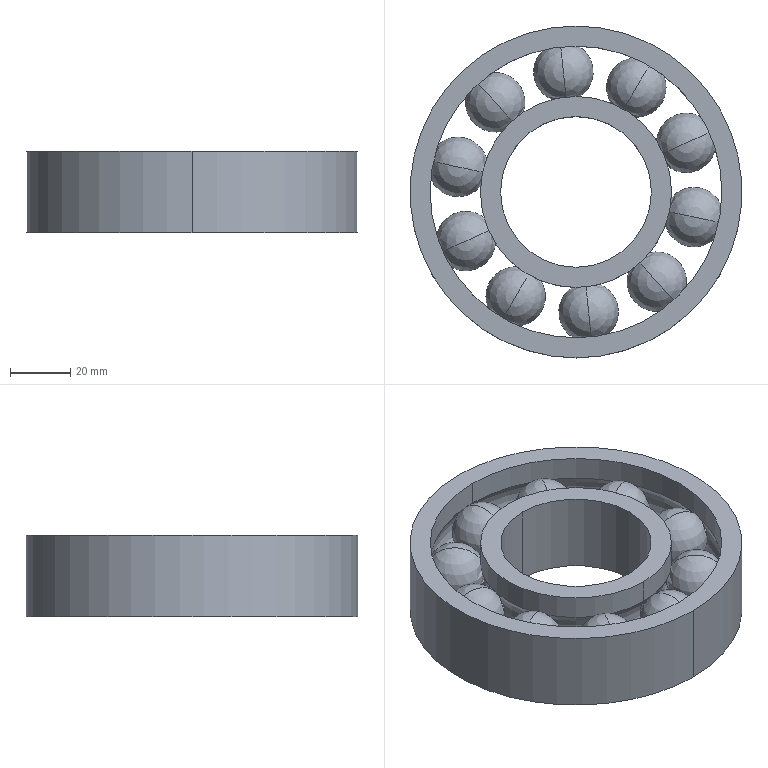Part | NX | features BREP 12 | 12 solids | 40 faces | box 110 x 110 x 27 mm | volume 126080 mm3 | sphere 20 | cylinder 12 | torus 4 | plane 4 | commonest cylinder face diameters 63.333 x4 96.667 x4 50 x2 110 x2
STEP:
#1=CARTESIAN_POINT('',(-26.765,29.726,-10.));
#2=VERTEX_POINT('',#1);
#3=CARTESIAN_POINT('',(-26.765,29.726,10.));
#4=VERTEX_POINT('',#3);
#5=CARTESIAN_POINT('',(-26.765,29.726,0.));
#6=DIRECTION('',(-0.7431,-0.6691,0.));
#7=DIRECTION('',(0.,0.,-1.));
#8=AXIS2_PLACEMENT_3D('',#5,#6,#7);
#9=CIRCLE('',#8,10.);
#10=EDGE_CURVE('',#2,#4,#9,.T.);
#11=ORIENTED_EDGE('',*,*,#10,.F.);
#12=CARTESIAN_POINT('',(-26.765,29.726,0.));
#13=DIRECTION('',(0.7431,0.6691,0.));
#14=DIRECTION('',(0.,0.,-1.));
#15=AXIS2_PLACEMENT_3D('',#12,#13,#14);
#16=CIRCLE('',#15,10.);
#17=EDGE_CURVE('',#2,#4,#16,.T.);
#18=ORIENTED_EDGE('',*,*,#17,.T.);
#19=EDGE_LOOP('',(#11,#18));
#20=FACE_BOUND('',#19,.T.);
#21=CARTESIAN_POINT('',(-26.765,29.726,0.));
#22=DIRECTION('',(0.,0.,-1.));
#23=DIRECTION('',(-0.6691,0.7431,0.));
#24=AXIS2_PLACEMENT_3D('',#21,#22,#23);
#25=SPHERICAL_SURFACE('',#24,10.);
#26=ADVANCED_FACE('',(#20),#25,.T.);
#27=ORIENTED_EDGE('',*,*,#10,.T.);
#28=ORIENTED_EDGE('',*,*,#17,.F.);
#29=EDGE_LOOP('',(#27,#28));
#30=FACE_BOUND('',#29,.T.);
#31=CARTESIAN_POINT('',(-26.765,29.726,0.));
#32=DIRECTION('',(0.,0.,-1.));
#33=DIRECTION('',(-0.6691,0.7431,0.));
#34=AXIS2_PLACEMENT_3D('',#31,#32,#33);
#35=SPHERICAL_SURFACE('',#34,10.);
#36=ADVANCED_FACE('',(#30),#35,.T.);
#37=CLOSED_SHELL('',(#26,#36));
#38=MANIFOLD_SOLID_BREP('',#37);
#39=CARTESIAN_POINT('',(36.542,16.269,10.));
#40=VERTEX_POINT('',#39);
#41=CARTESIAN_POINT('',(36.542,16.269,-10.));
#42=VERTEX_POINT('',#41);
#43=CARTESIAN_POINT('',(36.542,16.269,0.));
#44=DIRECTION('',(-0.4067,0.9135,0.));
#45=DIRECTION('',(0.,0.,-1.));
#46=AXIS2_PLACEMENT_3D('',#43,#44,#45);
#47=CIRCLE('',#46,10.);
#48=EDGE_CURVE('',#40,#42,#47,.F.);
#49=ORIENTED_EDGE('',*,*,#48,.T.);
#50=CARTESIAN_POINT('',(36.542,16.269,0.));
#51=DIRECTION('',(0.4067,-0.9135,0.));
#52=DIRECTION('',(0.,0.,-1.));
#53=AXIS2_PLACEMENT_3D('',#50,#51,#52);
#54=CIRCLE('',#53,10.);
#55=EDGE_CURVE('',#40,#42,#54,.F.);
#56=ORIENTED_EDGE('',*,*,#55,.F.);
#57=EDGE_LOOP('',(#49,#56));
#58=FACE_BOUND('',#57,.T.);
#59=CARTESIAN_POINT('',(36.542,16.269,0.));
#60=DIRECTION('',(0.,0.,-1.));
#61=DIRECTION('',(0.9135,0.4067,0.));
#62=AXIS2_PLACEMENT_3D('',#59,#60,#61);
#63=SPHERICAL_SURFACE('',#62,10.);
#64=ADVANCED_FACE('',(#58),#63,.T.);
#65=ORIENTED_EDGE('',*,*,#48,.F.);
#66=ORIENTED_EDGE('',*,*,#55,.T.);
#67=EDGE_LOOP('',(#65,#66));
#68=FACE_BOUND('',#67,.T.);
#69=CARTESIAN_POINT('',(36.542,16.269,0.));
#70=DIRECTION('',(0.,0.,-1.));
#71=DIRECTION('',(0.9135,0.4067,0.));
#72=AXIS2_PLACEMENT_3D('',#69,#70,#71);
#73=SPHERICAL_SURFACE('',#72,10.);
#74=ADVANCED_FACE('',(#68),#73,.T.);
#75=CLOSED_SHELL('',(#64,#74));
#76=MANIFOLD_SOLID_BREP('',#75);
#77=CARTESIAN_POINT('',(0.,31.667,5.528));
#78=VERTEX_POINT('',#77);
#79=CARTESIAN_POINT('',(0.,-31.667,5.528));
#80=VERTEX_POINT('',#79);
#81=CARTESIAN_POINT('',(0.,0.,5.528));
#82=DIRECTION('',(0.,0.,1.));
#83=DIRECTION('',(0.,1.,0.));
#84=AXIS2_PLACEMENT_3D('',#81,#82,#83);
#85=CIRCLE('',#84,31.667);
#86=EDGE_CURVE('',#78,#80,#85,.T.);
#87=ORIENTED_EDGE('',*,*,#86,.T.);
#88=CARTESIAN_POINT('',(0.,-31.667,13.5));
#89=VERTEX_POINT('',#88);
#90=CARTESIAN_POINT('',(0.,-31.667,5.528));
#91=DIRECTION('',(0.,0.,1.));
#92=VECTOR('',#91,1000.);
#93=LINE('',#90,#92);
#94=EDGE_CURVE('',#80,#89,#93,.T.);
#95=ORIENTED_EDGE('',*,*,#94,.T.);
#96=CARTESIAN_POINT('',(0.,31.667,13.5));
#97=VERTEX_POINT('',#96);
#98=CARTESIAN_POINT('',(0.,0.,13.5));
#99=DIRECTION('',(0.,0.,1.));
#100=DIRECTION('',(0.,1.,0.));
#101=AXIS2_PLACEMENT_3D('',#98,#99,#100);
#102=CIRCLE('',#101,31.667);
#103=EDGE_CURVE('',#97,#89,#102,.T.);
#104=ORIENTED_EDGE('',*,*,#103,.F.);
#105=CARTESIAN_POINT('',(0.,31.667,5.528));
#106=DIRECTION('',(0.,0.,1.));
#107=VECTOR('',#106,1000.);
#108=LINE('',#105,#107);
#109=EDGE_CURVE('',#78,#97,#108,.T.);
#110=ORIENTED_EDGE('',*,*,#109,.F.);
#111=EDGE_LOOP('',(#87,#95,#104,#110));
#112=FACE_BOUND('',#111,.T.);
#113=CARTESIAN_POINT('',(0.,0.,14.85));
#114=DIRECTION('',(0.,0.,-1.));
#115=DIRECTION('',(0.,1.,0.));
#116=AXIS2_PLACEMENT_3D('',#113,#114,#115);
#117=CYLINDRICAL_SURFACE('',#116,31.667);
#118=ADVANCED_FACE('',(#112),#117,.T.);
#119=CARTESIAN_POINT('',(0.,0.,13.5));
#120=DIRECTION('',(0.,0.,-1.));
#121=DIRECTION('',(0.,1.,0.));
#122=AXIS2_PLACEMENT_3D('',#119,#120,#121);
#123=CIRCLE('',#122,31.667);
#124=EDGE_CURVE('',#97,#89,#123,.T.);
#125=ORIENTED_EDGE('',*,*,#124,.T.);
#126=ORIENTED_EDGE('',*,*,#94,.F.);
#127=CARTESIAN_POINT('',(0.,0.,5.528));
#128=DIRECTION('',(0.,0.,-1.));
#129=DIRECTION('',(0.,1.,0.));
#130=AXIS2_PLACEMENT_3D('',#127,#128,#129);
#131=CIRCLE('',#130,31.667);
#132=EDGE_CURVE('',#78,#80,#131,.T.);
#133=ORIENTED_EDGE('',*,*,#132,.F.);
#134=ORIENTED_EDGE('',*,*,#109,.T.);
#135=EDGE_LOOP('',(#125,#126,#133,#134));
#136=FACE_BOUND('',#135,.T.);
#137=CARTESIAN_POINT('',(0.,0.,14.85));
#138=DIRECTION('',(0.,0.,-1.));
#139=DIRECTION('',(0.,1.,0.));
#140=AXIS2_PLACEMENT_3D('',#137,#138,#139);
#141=CYLINDRICAL_SURFACE('',#140,31.667);
#142=ADVANCED_FACE('',(#136),#141,.T.);
#143=ORIENTED_EDGE('',*,*,#132,.T.);
#144=CARTESIAN_POINT('',(0.,-31.667,-5.528));
#145=VERTEX_POINT('',#144);
#146=CARTESIAN_POINT('',(0.,-40.,0.));
#147=DIRECTION('',(1.,0.,0.));
#148=DIRECTION('',(0.,0.8333,-0.5528));
#149=AXIS2_PLACEMENT_3D('',#146,#147,#148);
#150=CIRCLE('',#149,10.);
#151=EDGE_CURVE('',#80,#145,#150,.F.);
#152=ORIENTED_EDGE('',*,*,#151,.T.);
#153=CARTESIAN_POINT('',(0.,31.667,-5.528));
#154=VERTEX_POINT('',#153);
#155=CARTESIAN_POINT('',(0.,0.,-5.528));
#156=DIRECTION('',(0.,0.,-1.));
#157=DIRECTION('',(0.,1.,0.));
#158=AXIS2_PLACEMENT_3D('',#155,#156,#157);
#159=CIRCLE('',#158,31.667);
#160=EDGE_CURVE('',#154,#145,#159,.T.);
#161=ORIENTED_EDGE('',*,*,#160,.F.);
#162=CARTESIAN_POINT('',(0.,40.,0.));
#163=DIRECTION('',(-1.,0.,0.));
#164=DIRECTION('',(0.,-0.8333,-0.5528));
#165=AXIS2_PLACEMENT_3D('',#162,#163,#164);
#166=CIRCLE('',#165,10.);
#167=EDGE_CURVE('',#78,#154,#166,.F.);
#168=ORIENTED_EDGE('',*,*,#167,.F.);
#169=EDGE_LOOP('',(#143,#152,#161,#168));
#170=FACE_BOUND('',#169,.T.);
#171=CARTESIAN_POINT('',(0.,0.,0.));
#172=DIRECTION('',(0.,0.,-1.));
#173=DIRECTION('',(0.,1.,0.));
#174=AXIS2_PLACEMENT_3D('',#171,#172,#173);
#175=TOROIDAL_SURFACE('',#174,40.,10.);
#176=ADVANCED_FACE('',(#170),#175,.F.);
#177=CARTESIAN_POINT('',(0.,0.,-5.528));
#178=DIRECTION('',(0.,0.,1.));
#179=DIRECTION('',(0.,1.,0.));
#180=AXIS2_PLACEMENT_3D('',#177,#178,#179);
#181=CIRCLE('',#180,31.667);
#182=EDGE_CURVE('',#154,#145,#181,.T.);
#183=ORIENTED_EDGE('',*,*,#182,.T.);
#184=ORIENTED_EDGE('',*,*,#151,.F.);
#185=ORIENTED_EDGE('',*,*,#86,.F.);
#186=ORIENTED_EDGE('',*,*,#167,.T.);
#187=EDGE_LOOP('',(#183,#184,#185,#186));
#188=FACE_BOUND('',#187,.T.);
#189=CARTESIAN_POINT('',(0.,0.,0.));
#190=DIRECTION('',(0.,0.,-1.));
#191=DIRECTION('',(0.,1.,0.));
#192=AXIS2_PLACEMENT_3D('',#189,#190,#191);
#193=TOROIDAL_SURFACE('',#192,40.,10.);
#194=ADVANCED_FACE('',(#188),#193,.F.);
#195=CARTESIAN_POINT('',(0.,31.667,-13.5));
#196=VERTEX_POINT('',#195);
#197=CARTESIAN_POINT('',(0.,-31.667,-13.5));
#198=VERTEX_POINT('',#197);
#199=CARTESIAN_POINT('',(0.,0.,-13.5));
#200=DIRECTION('',(0.,0.,1.));
#201=DIRECTION('',(0.,1.,0.));
#202=AXIS2_PLACEMENT_3D('',#199,#200,#201);
#203=CIRCLE('',#202,31.667);
#204=EDGE_CURVE('',#196,#198,#203,.T.);
#205=ORIENTED_EDGE('',*,*,#204,.T.);
#206=CARTESIAN_POINT('',(0.,-31.667,-13.5));
#207=DIRECTION('',(0.,0.,1.));
#208=VECTOR('',#207,1000.);
#209=LINE('',#206,#208);
#210=EDGE_CURVE('',#198,#145,#209,.T.);
#211=ORIENTED_EDGE('',*,*,#210,.T.);
#212=ORIENTED_EDGE('',*,*,#182,.F.);
#213=CARTESIAN_POINT('',(0.,31.667,-13.5));
#214=DIRECTION('',(0.,0.,1.));
#215=VECTOR('',#214,1000.);
#216=LINE('',#213,#215);
#217=EDGE_CURVE('',#196,#154,#216,.T.);
#218=ORIENTED_EDGE('',*,*,#217,.F.);
#219=EDGE_LOOP('',(#205,#211,#212,#218));
#220=FACE_BOUND('',#219,.T.);
#221=CARTESIAN_POINT('',(0.,0.,14.85));
#222=DIRECTION('',(0.,0.,-1.));
#223=DIRECTION('',(0.,1.,0.));
#224=AXIS2_PLACEMENT_3D('',#221,#222,#223);
#225=CYLINDRICAL_SURFACE('',#224,31.667);
#226=ADVANCED_FACE('',(#220),#225,.T.);
#227=ORIENTED_EDGE('',*,*,#160,.T.);
#228=ORIENTED_EDGE('',*,*,#210,.F.);
#229=CARTESIAN_POINT('',(0.,0.,-13.5));
#230=DIRECTION('',(0.,0.,-1.));
#231=DIRECTION('',(0.,1.,0.));
#232=AXIS2_PLACEMENT_3D('',#229,#230,#231);
#233=CIRCLE('',#232,31.667);
#234=EDGE_CURVE('',#196,#198,#233,.T.);
#235=ORIENTED_EDGE('',*,*,#234,.F.);
#236=ORIENTED_EDGE('',*,*,#217,.T.);
#237=EDGE_LOOP('',(#227,#228,#235,#236));
#238=FACE_BOUND('',#237,.T.);
#239=CARTESIAN_POINT('',(0.,0.,14.85));
#240=DIRECTION('',(0.,0.,-1.));
#241=DIRECTION('',(0.,1.,0.));
#242=AXIS2_PLACEMENT_3D('',#239,#240,#241);
#243=CYLINDRICAL_SURFACE('',#242,31.667);
#244=ADVANCED_FACE('',(#238),#243,.T.);
#245=ORIENTED_EDGE('',*,*,#204,.F.);
#246=ORIENTED_EDGE('',*,*,#234,.T.);
#247=EDGE_LOOP('',(#245,#246));
#248=FACE_BOUND('',#247,.T.);
#249=CARTESIAN_POINT('',(0.,25.,-13.5));
#250=VERTEX_POINT('',#249);
#251=CARTESIAN_POINT('',(0.,-25.,-13.5));
#252=VERTEX_POINT('',#251);
#253=CARTESIAN_POINT('',(0.,0.,-13.5));
#254=DIRECTION('',(0.,0.,-1.));
#255=DIRECTION('',(0.,1.,0.));
#256=AXIS2_PLACEMENT_3D('',#253,#254,#255);
#257=CIRCLE('',#256,25.);
#258=EDGE_CURVE('',#250,#252,#257,.T.);
#259=ORIENTED_EDGE('',*,*,#258,.F.);
#260=CARTESIAN_POINT('',(0.,0.,-13.5));
#261=DIRECTION('',(0.,0.,1.));
#262=DIRECTION('',(0.,1.,0.));
#263=AXIS2_PLACEMENT_3D('',#260,#261,#262);
#264=CIRCLE('',#263,25.);
#265=EDGE_CURVE('',#250,#252,#264,.T.);
#266=ORIENTED_EDGE('',*,*,#265,.T.);
#267=EDGE_LOOP('',(#259,#266));
#268=FACE_BOUND('',#267,.T.);
#269=CARTESIAN_POINT('',(0.,0.,-13.5));
#270=DIRECTION('',(0.,0.,-1.));
#271=DIRECTION('',(0.,1.,0.));
#272=AXIS2_PLACEMENT_3D('',#269,#270,#271);
#273=PLANE('',#272);
#274=ADVANCED_FACE('',(#248,#268),#273,.T.);
#275=CARTESIAN_POINT('',(0.,25.,13.5));
#276=VERTEX_POINT('',#275);
#277=CARTESIAN_POINT('',(0.,-25.,13.5));
#278=VERTEX_POINT('',#277);
#279=CARTESIAN_POINT('',(0.,0.,13.5));
#280=DIRECTION('',(0.,0.,1.));
#281=DIRECTION('',(0.,1.,0.));
#282=AXIS2_PLACEMENT_3D('',#279,#280,#281);
#283=CIRCLE('',#282,25.);
#284=EDGE_CURVE('',#276,#278,#283,.T.);
#285=ORIENTED_EDGE('',*,*,#284,.T.);
#286=CARTESIAN_POINT('',(0.,-25.,13.5));
#287=DIRECTION('',(0.,0.,-1.));
#288=VECTOR('',#287,1000.);
#289=LINE('',#286,#288);
#290=EDGE_CURVE('',#278,#252,#289,.T.);
#291=ORIENTED_EDGE('',*,*,#290,.T.);
#292=ORIENTED_EDGE('',*,*,#265,.F.);
#293=CARTESIAN_POINT('',(0.,25.,13.5));
#294=DIRECTION('',(0.,0.,-1.));
#295=VECTOR('',#294,1000.);
#296=LINE('',#293,#295);
#297=EDGE_CURVE('',#276,#250,#296,.T.);
#298=ORIENTED_EDGE('',*,*,#297,.F.);
#299=EDGE_LOOP('',(#285,#291,#292,#298));
#300=FACE_BOUND('',#299,.T.);
#301=CARTESIAN_POINT('',(0.,0.,14.85));
#302=DIRECTION('',(0.,0.,-1.));
#303=DIRECTION('',(0.,1.,0.));
#304=AXIS2_PLACEMENT_3D('',#301,#302,#303);
#305=CYLINDRICAL_SURFACE('',#304,25.);
#306=ADVANCED_FACE('',(#300),#305,.F.);
#307=ORIENTED_EDGE('',*,*,#258,.T.);
#308=ORIENTED_EDGE('',*,*,#290,.F.);
#309=CARTESIAN_POINT('',(0.,0.,13.5));
#310=DIRECTION('',(0.,0.,-1.));
#311=DIRECTION('',(0.,1.,0.));
#312=AXIS2_PLACEMENT_3D('',#309,#310,#311);
#313=CIRCLE('',#312,25.);
#314=EDGE_CURVE('',#276,#278,#313,.T.);
#315=ORIENTED_EDGE('',*,*,#314,.F.);
#316=ORIENTED_EDGE('',*,*,#297,.T.);
#317=EDGE_LOOP('',(#307,#308,#315,#316));
#318=FACE_BOUND('',#317,.T.);
#319=CARTESIAN_POINT('',(0.,0.,14.85));
#320=DIRECTION('',(0.,0.,-1.));
#321=DIRECTION('',(0.,1.,0.));
#322=AXIS2_PLACEMENT_3D('',#319,#320,#321);
#323=CYLINDRICAL_SURFACE('',#322,25.);
#324=ADVANCED_FACE('',(#318),#323,.F.);
#325=ORIENTED_EDGE('',*,*,#124,.F.);
#326=ORIENTED_EDGE('',*,*,#103,.T.);
#327=EDGE_LOOP('',(#325,#326));
#328=FACE_BOUND('',#327,.T.);
#329=ORIENTED_EDGE('',*,*,#284,.F.);
#330=ORIENTED_EDGE('',*,*,#314,.T.);
#331=EDGE_LOOP('',(#329,#330));
#332=FACE_BOUND('',#331,.T.);
#333=CARTESIAN_POINT('',(0.,0.,13.5));
#334=DIRECTION('',(0.,0.,-1.));
#335=DIRECTION('',(0.,1.,0.));
#336=AXIS2_PLACEMENT_3D('',#333,#334,#335);
#337=PLANE('',#336);
#338=ADVANCED_FACE('',(#328,#332),#337,.F.);
#339=CLOSED_SHELL('',(#118,#142,#176,#194,#226,#244,#274,#306,#324,#338));
#340=MANIFOLD_SOLID_BREP('',#339);
#341=CARTESIAN_POINT('',(26.765,-29.726,10.));
#342=VERTEX_POINT('',#341);
#343=CARTESIAN_POINT('',(26.765,-29.726,-10.));
#344=VERTEX_POINT('',#343);
#345=CARTESIAN_POINT('',(26.765,-29.726,0.));
#346=DIRECTION('',(0.7431,0.6691,0.));
#347=DIRECTION('',(0.,0.,-1.));
#348=AXIS2_PLACEMENT_3D('',#345,#346,#347);
#349=CIRCLE('',#348,10.);
#350=EDGE_CURVE('',#342,#344,#349,.F.);
#351=ORIENTED_EDGE('',*,*,#350,.T.);
#352=CARTESIAN_POINT('',(26.765,-29.726,0.));
#353=DIRECTION('',(-0.7431,-0.6691,0.));
#354=DIRECTION('',(0.,0.,-1.));
#355=AXIS2_PLACEMENT_3D('',#352,#353,#354);
#356=CIRCLE('',#355,10.);
#357=EDGE_CURVE('',#342,#344,#356,.F.);
#358=ORIENTED_EDGE('',*,*,#357,.F.);
#359=EDGE_LOOP('',(#351,#358));
#360=FACE_BOUND('',#359,.T.);
#361=CARTESIAN_POINT('',(26.765,-29.726,0.));
#362=DIRECTION('',(0.,0.,-1.));
#363=DIRECTION('',(0.6691,-0.7431,0.));
#364=AXIS2_PLACEMENT_3D('',#361,#362,#363);
#365=SPHERICAL_SURFACE('',#364,10.);
#366=ADVANCED_FACE('',(#360),#365,.T.);
#367=ORIENTED_EDGE('',*,*,#350,.F.);
#368=ORIENTED_EDGE('',*,*,#357,.T.);
#369=EDGE_LOOP('',(#367,#368));
#370=FACE_BOUND('',#369,.T.);
#371=CARTESIAN_POINT('',(26.765,-29.726,0.));
#372=DIRECTION('',(0.,0.,-1.));
#373=DIRECTION('',(0.6691,-0.7431,0.));
#374=AXIS2_PLACEMENT_3D('',#371,#372,#373);
#375=SPHERICAL_SURFACE('',#374,10.);
#376=ADVANCED_FACE('',(#370),#375,.T.);
#377=CLOSED_SHELL('',(#366,#376));
#378=MANIFOLD_SOLID_BREP('',#377);
#379=CARTESIAN_POINT('',(-20.,-34.641,-10.));
#380=VERTEX_POINT('',#379);
#381=CARTESIAN_POINT('',(-20.,-34.641,10.));
#382=VERTEX_POINT('',#381);
#383=CARTESIAN_POINT('',(-20.,-34.641,0.));
#384=DIRECTION('',(0.866,-0.5,0.));
#385=DIRECTION('',(0.,0.,-1.));
#386=AXIS2_PLACEMENT_3D('',#383,#384,#385);
#387=CIRCLE('',#386,10.);
#388=EDGE_CURVE('',#380,#382,#387,.T.);
#389=ORIENTED_EDGE('',*,*,#388,.F.);
#390=CARTESIAN_POINT('',(-20.,-34.641,0.));
#391=DIRECTION('',(-0.866,0.5,0.));
#392=DIRECTION('',(0.,0.,-1.));
#393=AXIS2_PLACEMENT_3D('',#390,#391,#392);
#394=CIRCLE('',#393,10.);
#395=EDGE_CURVE('',#380,#382,#394,.T.);
#396=ORIENTED_EDGE('',*,*,#395,.T.);
#397=EDGE_LOOP('',(#389,#396));
#398=FACE_BOUND('',#397,.T.);
#399=CARTESIAN_POINT('',(-20.,-34.641,0.));
#400=DIRECTION('',(0.,0.,-1.));
#401=DIRECTION('',(-0.5,-0.866,0.));
#402=AXIS2_PLACEMENT_3D('',#399,#400,#401);
#403=SPHERICAL_SURFACE('',#402,10.);
#404=ADVANCED_FACE('',(#398),#403,.T.);
#405=ORIENTED_EDGE('',*,*,#388,.T.);
#406=ORIENTED_EDGE('',*,*,#395,.F.);
#407=EDGE_LOOP('',(#405,#406));
#408=FACE_BOUND('',#407,.T.);
#409=CARTESIAN_POINT('',(-20.,-34.641,0.));
#410=DIRECTION('',(0.,0.,-1.));
#411=DIRECTION('',(-0.5,-0.866,0.));
#412=AXIS2_PLACEMENT_3D('',#409,#410,#411);
#413=SPHERICAL_SURFACE('',#412,10.);
#414=ADVANCED_FACE('',(#408),#413,.T.);
#415=CLOSED_SHELL('',(#404,#414));
#416=MANIFOLD_SOLID_BREP('',#415);
#417=CARTESIAN_POINT('',(0.,55.,-13.5));
#418=VERTEX_POINT('',#417);
#419=CARTESIAN_POINT('',(0.,-55.,-13.5));
#420=VERTEX_POINT('',#419);
#421=CARTESIAN_POINT('',(0.,0.,-13.5));
#422=DIRECTION('',(0.,0.,1.));
#423=DIRECTION('',(0.,1.,0.));
#424=AXIS2_PLACEMENT_3D('',#421,#422,#423);
#425=CIRCLE('',#424,55.);
#426=EDGE_CURVE('',#418,#420,#425,.T.);
#427=ORIENTED_EDGE('',*,*,#426,.T.);
#428=CARTESIAN_POINT('',(0.,-55.,13.5));
#429=VERTEX_POINT('',#428);
#430=CARTESIAN_POINT('',(0.,-55.,-13.5));
#431=DIRECTION('',(0.,0.,1.));
#432=VECTOR('',#431,1000.);
#433=LINE('',#430,#432);
#434=EDGE_CURVE('',#420,#429,#433,.T.);
#435=ORIENTED_EDGE('',*,*,#434,.T.);
#436=CARTESIAN_POINT('',(0.,55.,13.5));
#437=VERTEX_POINT('',#436);
#438=CARTESIAN_POINT('',(0.,0.,13.5));
#439=DIRECTION('',(0.,0.,1.));
#440=DIRECTION('',(0.,1.,0.));
#441=AXIS2_PLACEMENT_3D('',#438,#439,#440);
#442=CIRCLE('',#441,55.);
#443=EDGE_CURVE('',#437,#429,#442,.T.);
#444=ORIENTED_EDGE('',*,*,#443,.F.);
#445=CARTESIAN_POINT('',(0.,55.,-13.5));
#446=DIRECTION('',(0.,0.,1.));
#447=VECTOR('',#446,1000.);
#448=LINE('',#445,#447);
#449=EDGE_CURVE('',#418,#437,#448,.T.);
#450=ORIENTED_EDGE('',*,*,#449,.F.);
#451=EDGE_LOOP('',(#427,#435,#444,#450));
#452=FACE_BOUND('',#451,.T.);
#453=CARTESIAN_POINT('',(0.,0.,14.85));
#454=DIRECTION('',(0.,0.,-1.));
#455=DIRECTION('',(0.,1.,0.));
#456=AXIS2_PLACEMENT_3D('',#453,#454,#455);
#457=CYLINDRICAL_SURFACE('',#456,55.);
#458=ADVANCED_FACE('',(#452),#457,.T.);
#459=CARTESIAN_POINT('',(0.,0.,13.5));
#460=DIRECTION('',(0.,0.,-1.));
#461=DIRECTION('',(0.,1.,0.));
#462=AXIS2_PLACEMENT_3D('',#459,#460,#461);
#463=CIRCLE('',#462,55.);
#464=EDGE_CURVE('',#437,#429,#463,.T.);
#465=ORIENTED_EDGE('',*,*,#464,.T.);
#466=ORIENTED_EDGE('',*,*,#434,.F.);
#467=CARTESIAN_POINT('',(0.,0.,-13.5));
#468=DIRECTION('',(0.,0.,-1.));
#469=DIRECTION('',(0.,1.,0.));
#470=AXIS2_PLACEMENT_3D('',#467,#468,#469);
#471=CIRCLE('',#470,55.);
#472=EDGE_CURVE('',#418,#420,#471,.T.);
#473=ORIENTED_EDGE('',*,*,#472,.F.);
#474=ORIENTED_EDGE('',*,*,#449,.T.);
#475=EDGE_LOOP('',(#465,#466,#473,#474));
#476=FACE_BOUND('',#475,.T.);
#477=CARTESIAN_POINT('',(0.,0.,14.85));
#478=DIRECTION('',(0.,0.,-1.));
#479=DIRECTION('',(0.,1.,0.));
#480=AXIS2_PLACEMENT_3D('',#477,#478,#479);
#481=CYLINDRICAL_SURFACE('',#480,55.);
#482=ADVANCED_FACE('',(#476),#481,.T.);
#483=ORIENTED_EDGE('',*,*,#426,.F.);
#484=ORIENTED_EDGE('',*,*,#472,.T.);
#485=EDGE_LOOP('',(#483,#484));
#486=FACE_BOUND('',#485,.T.);
#487=CARTESIAN_POINT('',(0.,48.333,-13.5));
#488=VERTEX_POINT('',#487);
#489=CARTESIAN_POINT('',(0.,-48.333,-13.5));
#490=VERTEX_POINT('',#489);
#491=CARTESIAN_POINT('',(0.,0.,-13.5));
#492=DIRECTION('',(0.,0.,-1.));
#493=DIRECTION('',(0.,1.,0.));
#494=AXIS2_PLACEMENT_3D('',#491,#492,#493);
#495=CIRCLE('',#494,48.333);
#496=EDGE_CURVE('',#488,#490,#495,.T.);
#497=ORIENTED_EDGE('',*,*,#496,.F.);
#498=CARTESIAN_POINT('',(0.,0.,-13.5));
#499=DIRECTION('',(0.,0.,1.));
#500=DIRECTION('',(0.,1.,0.));
#501=AXIS2_PLACEMENT_3D('',#498,#499,#500);
#502=CIRCLE('',#501,48.333);
#503=EDGE_CURVE('',#488,#490,#502,.T.);
#504=ORIENTED_EDGE('',*,*,#503,.T.);
#505=EDGE_LOOP('',(#497,#504));
#506=FACE_BOUND('',#505,.T.);
#507=CARTESIAN_POINT('',(0.,0.,-13.5));
#508=DIRECTION('',(0.,0.,-1.));
#509=DIRECTION('',(0.,1.,0.));
#510=AXIS2_PLACEMENT_3D('',#507,#508,#509);
#511=PLANE('',#510);
#512=ADVANCED_FACE('',(#486,#506),#511,.T.);
#513=CARTESIAN_POINT('',(0.,48.333,-5.528));
#514=VERTEX_POINT('',#513);
#515=CARTESIAN_POINT('',(0.,-48.333,-5.528));
#516=VERTEX_POINT('',#515);
#517=CARTESIAN_POINT('',(0.,0.,-5.528));
#518=DIRECTION('',(0.,0.,1.));
#519=DIRECTION('',(0.,1.,0.));
#520=AXIS2_PLACEMENT_3D('',#517,#518,#519);
#521=CIRCLE('',#520,48.333);
#522=EDGE_CURVE('',#514,#516,#521,.T.);
#523=ORIENTED_EDGE('',*,*,#522,.T.);
#524=CARTESIAN_POINT('',(0.,-48.333,-5.528));
#525=DIRECTION('',(0.,0.,-1.));
#526=VECTOR('',#525,1000.);
#527=LINE('',#524,#526);
#528=EDGE_CURVE('',#516,#490,#527,.T.);
#529=ORIENTED_EDGE('',*,*,#528,.T.);
#530=ORIENTED_EDGE('',*,*,#503,.F.);
#531=CARTESIAN_POINT('',(0.,48.333,-5.528));
#532=DIRECTION('',(0.,0.,-1.));
#533=VECTOR('',#532,1000.);
#534=LINE('',#531,#533);
#535=EDGE_CURVE('',#514,#488,#534,.T.);
#536=ORIENTED_EDGE('',*,*,#535,.F.);
#537=EDGE_LOOP('',(#523,#529,#530,#536));
#538=FACE_BOUND('',#537,.T.);
#539=CARTESIAN_POINT('',(0.,0.,14.85));
#540=DIRECTION('',(0.,0.,-1.));
#541=DIRECTION('',(0.,1.,0.));
#542=AXIS2_PLACEMENT_3D('',#539,#540,#541);
#543=CYLINDRICAL_SURFACE('',#542,48.333);
#544=ADVANCED_FACE('',(#538),#543,.F.);
#545=ORIENTED_EDGE('',*,*,#496,.T.);
#546=ORIENTED_EDGE('',*,*,#528,.F.);
#547=CARTESIAN_POINT('',(0.,0.,-5.528));
#548=DIRECTION('',(0.,0.,-1.));
#549=DIRECTION('',(0.,1.,0.));
#550=AXIS2_PLACEMENT_3D('',#547,#548,#549);
#551=CIRCLE('',#550,48.333);
#552=EDGE_CURVE('',#514,#516,#551,.T.);
#553=ORIENTED_EDGE('',*,*,#552,.F.);
#554=ORIENTED_EDGE('',*,*,#535,.T.);
#555=EDGE_LOOP('',(#545,#546,#553,#554));
#556=FACE_BOUND('',#555,.T.);
#557=CARTESIAN_POINT('',(0.,0.,14.85));
#558=DIRECTION('',(0.,0.,-1.));
#559=DIRECTION('',(0.,1.,0.));
#560=AXIS2_PLACEMENT_3D('',#557,#558,#559);
#561=CYLINDRICAL_SURFACE('',#560,48.333);
#562=ADVANCED_FACE('',(#556),#561,.F.);
#563=ORIENTED_EDGE('',*,*,#552,.T.);
#564=CARTESIAN_POINT('',(0.,-48.333,5.528));
#565=VERTEX_POINT('',#564);
#566=CARTESIAN_POINT('',(0.,-40.,0.));
#567=DIRECTION('',(1.,0.,0.));
#568=DIRECTION('',(0.,-0.8333,0.5528));
#569=AXIS2_PLACEMENT_3D('',#566,#567,#568);
#570=CIRCLE('',#569,10.);
#571=EDGE_CURVE('',#516,#565,#570,.F.);
#572=ORIENTED_EDGE('',*,*,#571,.T.);
#573=CARTESIAN_POINT('',(0.,48.333,5.528));
#574=VERTEX_POINT('',#573);
#575=CARTESIAN_POINT('',(0.,0.,5.528));
#576=DIRECTION('',(0.,0.,-1.));
#577=DIRECTION('',(0.,1.,0.));
#578=AXIS2_PLACEMENT_3D('',#575,#576,#577);
#579=CIRCLE('',#578,48.333);
#580=EDGE_CURVE('',#574,#565,#579,.T.);
#581=ORIENTED_EDGE('',*,*,#580,.F.);
#582=CARTESIAN_POINT('',(0.,40.,0.));
#583=DIRECTION('',(-1.,0.,0.));
#584=DIRECTION('',(0.,0.8333,0.5528));
#585=AXIS2_PLACEMENT_3D('',#582,#583,#584);
#586=CIRCLE('',#585,10.);
#587=EDGE_CURVE('',#514,#574,#586,.F.);
#588=ORIENTED_EDGE('',*,*,#587,.F.);
#589=EDGE_LOOP('',(#563,#572,#581,#588));
#590=FACE_BOUND('',#589,.T.);
#591=CARTESIAN_POINT('',(0.,0.,0.));
#592=DIRECTION('',(0.,0.,-1.));
#593=DIRECTION('',(0.,1.,0.));
#594=AXIS2_PLACEMENT_3D('',#591,#592,#593);
#595=TOROIDAL_SURFACE('',#594,40.,10.);
#596=ADVANCED_FACE('',(#590),#595,.F.);
#597=CARTESIAN_POINT('',(0.,0.,5.528));
#598=DIRECTION('',(0.,0.,1.));
#599=DIRECTION('',(0.,1.,0.));
#600=AXIS2_PLACEMENT_3D('',#597,#598,#599);
#601=CIRCLE('',#600,48.333);
#602=EDGE_CURVE('',#574,#565,#601,.T.);
#603=ORIENTED_EDGE('',*,*,#602,.T.);
#604=ORIENTED_EDGE('',*,*,#571,.F.);
#605=ORIENTED_EDGE('',*,*,#522,.F.);
#606=ORIENTED_EDGE('',*,*,#587,.T.);
#607=EDGE_LOOP('',(#603,#604,#605,#606));
#608=FACE_BOUND('',#607,.T.);
#609=CARTESIAN_POINT('',(0.,0.,0.));
#610=DIRECTION('',(0.,0.,-1.));
#611=DIRECTION('',(0.,1.,0.));
#612=AXIS2_PLACEMENT_3D('',#609,#610,#611);
#613=TOROIDAL_SURFACE('',#612,40.,10.);
#614=ADVANCED_FACE('',(#608),#613,.F.);
#615=CARTESIAN_POINT('',(0.,48.333,13.5));
#616=VERTEX_POINT('',#615);
#617=CARTESIAN_POINT('',(0.,-48.333,13.5));
#618=VERTEX_POINT('',#617);
#619=CARTESIAN_POINT('',(0.,0.,13.5));
#620=DIRECTION('',(0.,0.,1.));
#621=DIRECTION('',(0.,1.,0.));
#622=AXIS2_PLACEMENT_3D('',#619,#620,#621);
#623=CIRCLE('',#622,48.333);
#624=EDGE_CURVE('',#616,#618,#623,.T.);
#625=ORIENTED_EDGE('',*,*,#624,.T.);
#626=CARTESIAN_POINT('',(0.,-48.333,13.5));
#627=DIRECTION('',(0.,0.,-1.));
#628=VECTOR('',#627,1000.);
#629=LINE('',#626,#628);
#630=EDGE_CURVE('',#618,#565,#629,.T.);
#631=ORIENTED_EDGE('',*,*,#630,.T.);
#632=ORIENTED_EDGE('',*,*,#602,.F.);
#633=CARTESIAN_POINT('',(0.,48.333,13.5));
#634=DIRECTION('',(0.,0.,-1.));
#635=VECTOR('',#634,1000.);
#636=LINE('',#633,#635);
#637=EDGE_CURVE('',#616,#574,#636,.T.);
#638=ORIENTED_EDGE('',*,*,#637,.F.);
#639=EDGE_LOOP('',(#625,#631,#632,#638));
#640=FACE_BOUND('',#639,.T.);
#641=CARTESIAN_POINT('',(0.,0.,14.85));
#642=DIRECTION('',(0.,0.,-1.));
#643=DIRECTION('',(0.,1.,0.));
#644=AXIS2_PLACEMENT_3D('',#641,#642,#643);
#645=CYLINDRICAL_SURFACE('',#644,48.333);
#646=ADVANCED_FACE('',(#640),#645,.F.);
#647=ORIENTED_EDGE('',*,*,#580,.T.);
#648=ORIENTED_EDGE('',*,*,#630,.F.);
#649=CARTESIAN_POINT('',(0.,0.,13.5));
#650=DIRECTION('',(0.,0.,-1.));
#651=DIRECTION('',(0.,1.,0.));
#652=AXIS2_PLACEMENT_3D('',#649,#650,#651);
#653=CIRCLE('',#652,48.333);
#654=EDGE_CURVE('',#616,#618,#653,.T.);
#655=ORIENTED_EDGE('',*,*,#654,.F.);
#656=ORIENTED_EDGE('',*,*,#637,.T.);
#657=EDGE_LOOP('',(#647,#648,#655,#656));
#658=FACE_BOUND('',#657,.T.);
#659=CARTESIAN_POINT('',(0.,0.,14.85));
#660=DIRECTION('',(0.,0.,-1.));
#661=DIRECTION('',(0.,1.,0.));
#662=AXIS2_PLACEMENT_3D('',#659,#660,#661);
#663=CYLINDRICAL_SURFACE('',#662,48.333);
#664=ADVANCED_FACE('',(#658),#663,.F.);
#665=ORIENTED_EDGE('',*,*,#464,.F.);
#666=ORIENTED_EDGE('',*,*,#443,.T.);
#667=EDGE_LOOP('',(#665,#666));
#668=FACE_BOUND('',#667,.T.);
#669=ORIENTED_EDGE('',*,*,#624,.F.);
#670=ORIENTED_EDGE('',*,*,#654,.T.);
#671=EDGE_LOOP('',(#669,#670));
#672=FACE_BOUND('',#671,.T.);
#673=CARTESIAN_POINT('',(0.,0.,13.5));
#674=DIRECTION('',(0.,0.,-1.));
#675=DIRECTION('',(0.,1.,0.));
#676=AXIS2_PLACEMENT_3D('',#673,#674,#675);
#677=PLANE('',#676);
#678=ADVANCED_FACE('',(#668,#672),#677,.F.);
#679=CLOSED_SHELL('',(#458,#482,#512,#544,#562,#596,#614,#646,#664,#678));
#680=MANIFOLD_SOLID_BREP('',#679);
#681=CARTESIAN_POINT('',(39.126,-8.316,10.));
#682=VERTEX_POINT('',#681);
#683=CARTESIAN_POINT('',(39.126,-8.316,-10.));
#684=VERTEX_POINT('',#683);
#685=CARTESIAN_POINT('',(39.126,-8.316,0.));
#686=DIRECTION('',(0.2079,0.9781,0.));
#687=DIRECTION('',(0.,0.,-1.));
#688=AXIS2_PLACEMENT_3D('',#685,#686,#687);
#689=CIRCLE('',#688,10.);
#690=EDGE_CURVE('',#682,#684,#689,.F.);
#691=ORIENTED_EDGE('',*,*,#690,.T.);
#692=CARTESIAN_POINT('',(39.126,-8.316,0.));
#693=DIRECTION('',(-0.2079,-0.9781,0.));
#694=DIRECTION('',(0.,0.,-1.));
#695=AXIS2_PLACEMENT_3D('',#692,#693,#694);
#696=CIRCLE('',#695,10.);
#697=EDGE_CURVE('',#682,#684,#696,.F.);
#698=ORIENTED_EDGE('',*,*,#697,.F.);
#699=EDGE_LOOP('',(#691,#698));
#700=FACE_BOUND('',#699,.T.);
#701=CARTESIAN_POINT('',(39.126,-8.316,0.));
#702=DIRECTION('',(0.,0.,-1.));
#703=DIRECTION('',(0.9781,-0.2079,0.));
#704=AXIS2_PLACEMENT_3D('',#701,#702,#703);
#705=SPHERICAL_SURFACE('',#704,10.);
#706=ADVANCED_FACE('',(#700),#705,.T.);
#707=ORIENTED_EDGE('',*,*,#690,.F.);
#708=ORIENTED_EDGE('',*,*,#697,.T.);
#709=EDGE_LOOP('',(#707,#708));
#710=FACE_BOUND('',#709,.T.);
#711=CARTESIAN_POINT('',(39.126,-8.316,0.));
#712=DIRECTION('',(0.,0.,-1.));
#713=DIRECTION('',(0.9781,-0.2079,0.));
#714=AXIS2_PLACEMENT_3D('',#711,#712,#713);
#715=SPHERICAL_SURFACE('',#714,10.);
#716=ADVANCED_FACE('',(#710),#715,.T.);
#717=CLOSED_SHELL('',(#706,#716));
#718=MANIFOLD_SOLID_BREP('',#717);
#719=CARTESIAN_POINT('',(-39.126,8.316,-10.));
#720=VERTEX_POINT('',#719);
#721=CARTESIAN_POINT('',(-39.126,8.316,10.));
#722=VERTEX_POINT('',#721);
#723=CARTESIAN_POINT('',(-39.126,8.316,0.));
#724=DIRECTION('',(-0.2079,-0.9781,0.));
#725=DIRECTION('',(0.,0.,-1.));
#726=AXIS2_PLACEMENT_3D('',#723,#724,#725);
#727=CIRCLE('',#726,10.);
#728=EDGE_CURVE('',#720,#722,#727,.T.);
#729=ORIENTED_EDGE('',*,*,#728,.F.);
#730=CARTESIAN_POINT('',(-39.126,8.316,0.));
#731=DIRECTION('',(0.2079,0.9781,0.));
#732=DIRECTION('',(0.,0.,-1.));
#733=AXIS2_PLACEMENT_3D('',#730,#731,#732);
#734=CIRCLE('',#733,10.);
#735=EDGE_CURVE('',#720,#722,#734,.T.);
#736=ORIENTED_EDGE('',*,*,#735,.T.);
#737=EDGE_LOOP('',(#729,#736));
#738=FACE_BOUND('',#737,.T.);
#739=CARTESIAN_POINT('',(-39.126,8.316,0.));
#740=DIRECTION('',(0.,0.,-1.));
#741=DIRECTION('',(-0.9781,0.2079,0.));
#742=AXIS2_PLACEMENT_3D('',#739,#740,#741);
#743=SPHERICAL_SURFACE('',#742,10.);
#744=ADVANCED_FACE('',(#738),#743,.T.);
#745=ORIENTED_EDGE('',*,*,#728,.T.);
#746=ORIENTED_EDGE('',*,*,#735,.F.);
#747=EDGE_LOOP('',(#745,#746));
#748=FACE_BOUND('',#747,.T.);
#749=CARTESIAN_POINT('',(-39.126,8.316,0.));
#750=DIRECTION('',(0.,0.,-1.));
#751=DIRECTION('',(-0.9781,0.2079,0.));
#752=AXIS2_PLACEMENT_3D('',#749,#750,#751);
#753=SPHERICAL_SURFACE('',#752,10.);
#754=ADVANCED_FACE('',(#748),#753,.T.);
#755=CLOSED_SHELL('',(#744,#754));
#756=MANIFOLD_SOLID_BREP('',#755);
#757=CARTESIAN_POINT('',(4.181,-39.781,10.));
#758=VERTEX_POINT('',#757);
#759=CARTESIAN_POINT('',(4.181,-39.781,-10.));
#760=VERTEX_POINT('',#759);
#761=CARTESIAN_POINT('',(4.181,-39.781,0.));
#762=DIRECTION('',(0.9945,0.1045,0.));
#763=DIRECTION('',(0.,0.,-1.));
#764=AXIS2_PLACEMENT_3D('',#761,#762,#763);
#765=CIRCLE('',#764,10.);
#766=EDGE_CURVE('',#758,#760,#765,.F.);
#767=ORIENTED_EDGE('',*,*,#766,.T.);
#768=CARTESIAN_POINT('',(4.181,-39.781,0.));
#769=DIRECTION('',(-0.9945,-0.1045,0.));
#770=DIRECTION('',(0.,0.,-1.));
#771=AXIS2_PLACEMENT_3D('',#768,#769,#770);
#772=CIRCLE('',#771,10.);
#773=EDGE_CURVE('',#758,#760,#772,.F.);
#774=ORIENTED_EDGE('',*,*,#773,.F.);
#775=EDGE_LOOP('',(#767,#774));
#776=FACE_BOUND('',#775,.T.);
#777=CARTESIAN_POINT('',(4.181,-39.781,0.));
#778=DIRECTION('',(0.,0.,-1.));
#779=DIRECTION('',(0.1045,-0.9945,0.));
#780=AXIS2_PLACEMENT_3D('',#777,#778,#779);
#781=SPHERICAL_SURFACE('',#780,10.);
#782=ADVANCED_FACE('',(#776),#781,.T.);
#783=ORIENTED_EDGE('',*,*,#766,.F.);
#784=ORIENTED_EDGE('',*,*,#773,.T.);
#785=EDGE_LOOP('',(#783,#784));
#786=FACE_BOUND('',#785,.T.);
#787=CARTESIAN_POINT('',(4.181,-39.781,0.));
#788=DIRECTION('',(0.,0.,-1.));
#789=DIRECTION('',(0.1045,-0.9945,0.));
#790=AXIS2_PLACEMENT_3D('',#787,#788,#789);
#791=SPHERICAL_SURFACE('',#790,10.);
#792=ADVANCED_FACE('',(#786),#791,.T.);
#793=CLOSED_SHELL('',(#782,#792));
#794=MANIFOLD_SOLID_BREP('',#793);
#795=CARTESIAN_POINT('',(20.,34.641,10.));
#796=VERTEX_POINT('',#795);
#797=CARTESIAN_POINT('',(20.,34.641,-10.));
#798=VERTEX_POINT('',#797);
#799=CARTESIAN_POINT('',(20.,34.641,0.));
#800=DIRECTION('',(-0.866,0.5,0.));
#801=DIRECTION('',(0.,0.,-1.));
#802=AXIS2_PLACEMENT_3D('',#799,#800,#801);
#803=CIRCLE('',#802,10.);
#804=EDGE_CURVE('',#796,#798,#803,.F.);
#805=ORIENTED_EDGE('',*,*,#804,.T.);
#806=CARTESIAN_POINT('',(20.,34.641,0.));
#807=DIRECTION('',(0.866,-0.5,0.));
#808=DIRECTION('',(0.,0.,-1.));
#809=AXIS2_PLACEMENT_3D('',#806,#807,#808);
#810=CIRCLE('',#809,10.);
#811=EDGE_CURVE('',#796,#798,#810,.F.);
#812=ORIENTED_EDGE('',*,*,#811,.F.);
#813=EDGE_LOOP('',(#805,#812));
#814=FACE_BOUND('',#813,.T.);
#815=CARTESIAN_POINT('',(20.,34.641,0.));
#816=DIRECTION('',(0.,0.,-1.));
#817=DIRECTION('',(0.5,0.866,0.));
#818=AXIS2_PLACEMENT_3D('',#815,#816,#817);
#819=SPHERICAL_SURFACE('',#818,10.);
#820=ADVANCED_FACE('',(#814),#819,.T.);
#821=ORIENTED_EDGE('',*,*,#804,.F.);
#822=ORIENTED_EDGE('',*,*,#811,.T.);
#823=EDGE_LOOP('',(#821,#822));
#824=FACE_BOUND('',#823,.T.);
#825=CARTESIAN_POINT('',(20.,34.641,0.));
#826=DIRECTION('',(0.,0.,-1.));
#827=DIRECTION('',(0.5,0.866,0.));
#828=AXIS2_PLACEMENT_3D('',#825,#826,#827);
#829=SPHERICAL_SURFACE('',#828,10.);
#830=ADVANCED_FACE('',(#824),#829,.T.);
#831=CLOSED_SHELL('',(#820,#830));
#832=MANIFOLD_SOLID_BREP('',#831);
#833=CARTESIAN_POINT('',(-36.542,-16.269,-10.));
#834=VERTEX_POINT('',#833);
#835=CARTESIAN_POINT('',(-36.542,-16.269,10.));
#836=VERTEX_POINT('',#835);
#837=CARTESIAN_POINT('',(-36.542,-16.269,0.));
#838=DIRECTION('',(0.4067,-0.9135,0.));
#839=DIRECTION('',(0.,0.,-1.));
#840=AXIS2_PLACEMENT_3D('',#837,#838,#839);
#841=CIRCLE('',#840,10.);
#842=EDGE_CURVE('',#834,#836,#841,.T.);
#843=ORIENTED_EDGE('',*,*,#842,.F.);
#844=CARTESIAN_POINT('',(-36.542,-16.269,0.));
#845=DIRECTION('',(-0.4067,0.9135,0.));
#846=DIRECTION('',(0.,0.,-1.));
#847=AXIS2_PLACEMENT_3D('',#844,#845,#846);
#848=CIRCLE('',#847,10.);
#849=EDGE_CURVE('',#834,#836,#848,.T.);
#850=ORIENTED_EDGE('',*,*,#849,.T.);
#851=EDGE_LOOP('',(#843,#850));
#852=FACE_BOUND('',#851,.T.);
#853=CARTESIAN_POINT('',(-36.542,-16.269,0.));
#854=DIRECTION('',(0.,0.,-1.));
#855=DIRECTION('',(-0.9135,-0.4067,0.));
#856=AXIS2_PLACEMENT_3D('',#853,#854,#855);
#857=SPHERICAL_SURFACE('',#856,10.);
#858=ADVANCED_FACE('',(#852),#857,.T.);
#859=ORIENTED_EDGE('',*,*,#842,.T.);
#860=ORIENTED_EDGE('',*,*,#849,.F.);
#861=EDGE_LOOP('',(#859,#860));
#862=FACE_BOUND('',#861,.T.);
#863=CARTESIAN_POINT('',(-36.542,-16.269,0.));
#864=DIRECTION('',(0.,0.,-1.));
#865=DIRECTION('',(-0.9135,-0.4067,0.));
#866=AXIS2_PLACEMENT_3D('',#863,#864,#865);
#867=SPHERICAL_SURFACE('',#866,10.);
#868=ADVANCED_FACE('',(#862),#867,.T.);
#869=CLOSED_SHELL('',(#858,#868));
#870=MANIFOLD_SOLID_BREP('',#869);
#871=CARTESIAN_POINT('',(-4.181,39.781,-10.));
#872=VERTEX_POINT('',#871);
#873=CARTESIAN_POINT('',(-4.181,39.781,10.));
#874=VERTEX_POINT('',#873);
#875=CARTESIAN_POINT('',(-4.181,39.781,0.));
#876=DIRECTION('',(-0.9945,-0.1045,0.));
#877=DIRECTION('',(0.,0.,-1.));
#878=AXIS2_PLACEMENT_3D('',#875,#876,#877);
#879=CIRCLE('',#878,10.);
#880=EDGE_CURVE('',#872,#874,#879,.T.);
#881=ORIENTED_EDGE('',*,*,#880,.F.);
#882=CARTESIAN_POINT('',(-4.181,39.781,0.));
#883=DIRECTION('',(0.9945,0.1045,0.));
#884=DIRECTION('',(0.,0.,-1.));
#885=AXIS2_PLACEMENT_3D('',#882,#883,#884);
#886=CIRCLE('',#885,10.);
#887=EDGE_CURVE('',#872,#874,#886,.T.);
#888=ORIENTED_EDGE('',*,*,#887,.T.);
#889=EDGE_LOOP('',(#881,#888));
#890=FACE_BOUND('',#889,.T.);
#891=CARTESIAN_POINT('',(-4.181,39.781,0.));
#892=DIRECTION('',(0.,0.,-1.));
#893=DIRECTION('',(-0.1045,0.9945,0.));
#894=AXIS2_PLACEMENT_3D('',#891,#892,#893);
#895=SPHERICAL_SURFACE('',#894,10.);
#896=ADVANCED_FACE('',(#890),#895,.T.);
#897=ORIENTED_EDGE('',*,*,#880,.T.);
#898=ORIENTED_EDGE('',*,*,#887,.F.);
#899=EDGE_LOOP('',(#897,#898));
#900=FACE_BOUND('',#899,.T.);
#901=CARTESIAN_POINT('',(-4.181,39.781,0.));
#902=DIRECTION('',(0.,0.,-1.));
#903=DIRECTION('',(-0.1045,0.9945,0.));
#904=AXIS2_PLACEMENT_3D('',#901,#902,#903);
#905=SPHERICAL_SURFACE('',#904,10.);
#906=ADVANCED_FACE('',(#900),#905,.T.);
#907=CLOSED_SHELL('',(#896,#906));
#908=MANIFOLD_SOLID_BREP('',#907);
#909=(LENGTH_UNIT()NAMED_UNIT(*)SI_UNIT(.MILLI.,.METRE.));
#910=UNCERTAINTY_MEASURE_WITH_UNIT(LENGTH_MEASURE(0.00001),#909,'','');
#911=(NAMED_UNIT(*)PLANE_ANGLE_UNIT()SI_UNIT($,.RADIAN.));
#912=(NAMED_UNIT(*)SI_UNIT($,.STERADIAN.)SOLID_ANGLE_UNIT());
#913=(GEOMETRIC_REPRESENTATION_CONTEXT(3)GLOBAL_UNCERTAINTY_ASSIGNED_CONTEXT((#910))GLOBAL_UNIT_ASSIGNED_CONTEXT((#909,#911,#912))REPRESENTATION_CONTEXT('',''));
#914=ADVANCED_BREP_SHAPE_REPRESENTATION('',(#38,#76,#340,#378,#416,#680,#718,#756,#794,#832,#870,#908),#913);